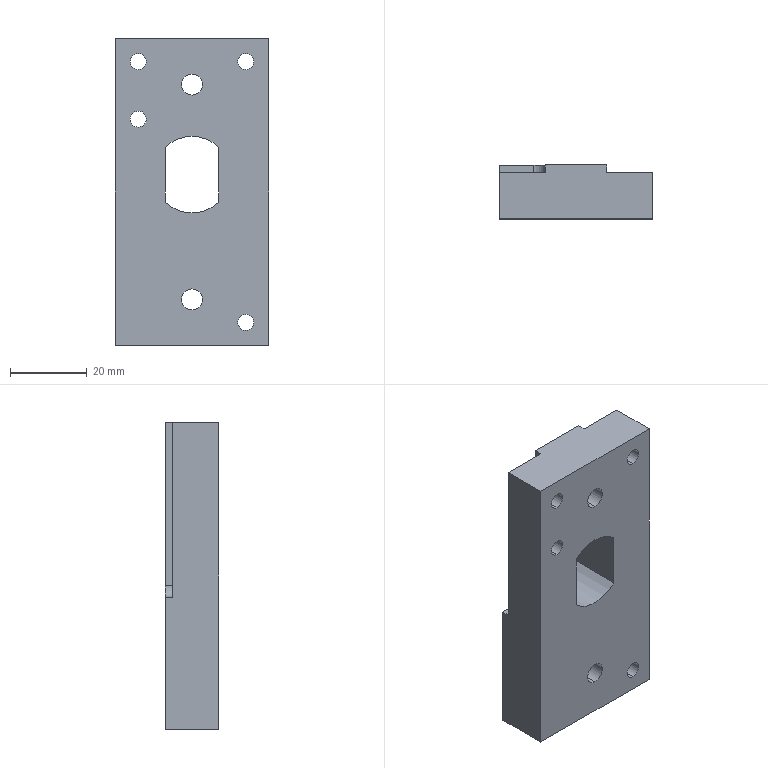Part | STEP file | detection track | 1 solid | 35 faces | box 40 x 14 x 80 mm | volume 36343 mm3 | cylinder 20 | plane 15 | commonest cylinder face diameters 4.2 x8 5.5 x4 10 x4 20 x3 6 x1